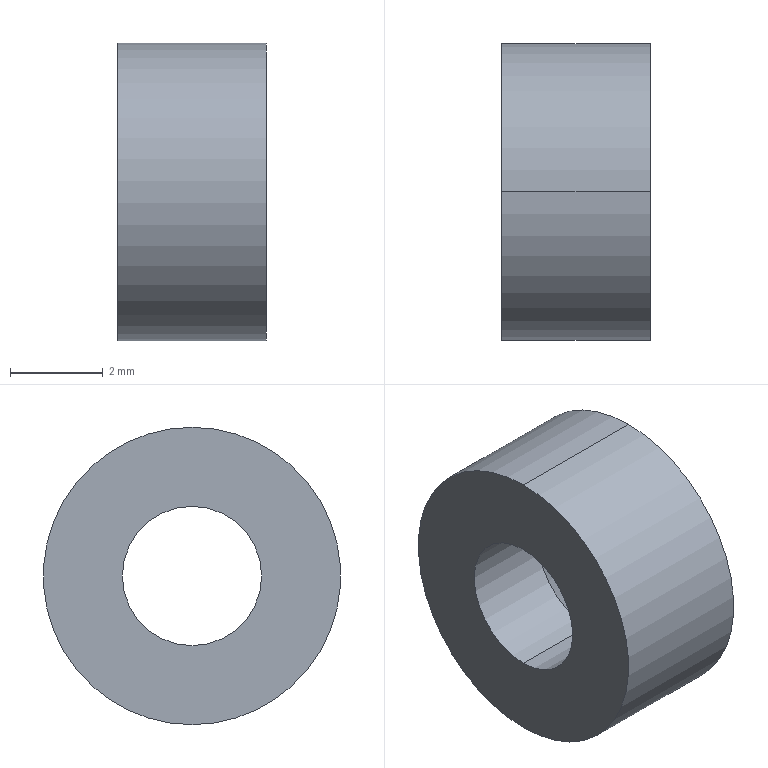Part | STEP file | 11-FG99-HXCC8magnet-V3.0-kkkkkk-998.11 | 1 solid | 8 faces | box 3.2 x 6.4 x 6.4 mm | volume 70.916 mm3 | cylinder 4 | cone 2 | plane 2 | commonest cylinder face diameters 3 x2 6.4 x2
STEP:
#1=CARTESIAN_POINT('',(3.8,0.,3.2));
#2=VERTEX_POINT('',#1);
#3=CARTESIAN_POINT('',(3.8,0.,-3.2));
#4=VERTEX_POINT('',#3);
#5=CARTESIAN_POINT('',(3.8,0.,0.));
#6=DIRECTION('',(-1.,0.,0.));
#7=DIRECTION('',(0.,0.,1.));
#8=AXIS2_PLACEMENT_3D('',#5,#6,#7);
#9=CIRCLE('',#8,3.2);
#10=EDGE_CURVE('',#2,#4,#9,.T.);
#11=ORIENTED_EDGE('',*,*,#10,.T.);
#12=CARTESIAN_POINT('',(0.6,0.,-3.2));
#13=VERTEX_POINT('',#12);
#14=CARTESIAN_POINT('',(4.,0.,-3.2));
#15=DIRECTION('',(-1.,0.,0.));
#16=VECTOR('',#15,1000.);
#17=LINE('',#14,#16);
#18=EDGE_CURVE('',#4,#13,#17,.T.);
#19=ORIENTED_EDGE('',*,*,#18,.T.);
#20=CARTESIAN_POINT('',(0.6,0.,3.2));
#21=VERTEX_POINT('',#20);
#22=CARTESIAN_POINT('',(0.6,0.,0.));
#23=DIRECTION('',(-1.,0.,0.));
#24=DIRECTION('',(0.,0.,1.));
#25=AXIS2_PLACEMENT_3D('',#22,#23,#24);
#26=CIRCLE('',#25,3.2);
#27=EDGE_CURVE('',#21,#13,#26,.T.);
#28=ORIENTED_EDGE('',*,*,#27,.F.);
#29=CARTESIAN_POINT('',(4.,0.,3.2));
#30=DIRECTION('',(-1.,0.,0.));
#31=VECTOR('',#30,1000.);
#32=LINE('',#29,#31);
#33=EDGE_CURVE('',#2,#21,#32,.T.);
#34=ORIENTED_EDGE('',*,*,#33,.F.);
#35=EDGE_LOOP('',(#11,#19,#28,#34));
#36=FACE_OUTER_BOUND('',#35,.T.);
#37=CARTESIAN_POINT('',(4.,0.,0.));
#38=DIRECTION('',(-1.,0.,0.));
#39=DIRECTION('',(0.,0.,1.));
#40=AXIS2_PLACEMENT_3D('',#37,#38,#39);
#41=CYLINDRICAL_SURFACE('',#40,3.2);
#42=ADVANCED_FACE('',(#36),#41,.T.);
#43=CARTESIAN_POINT('',(2.55,0.,-1.5));
#44=VERTEX_POINT('',#43);
#45=CARTESIAN_POINT('',(2.55,0.,1.5));
#46=VERTEX_POINT('',#45);
#47=CARTESIAN_POINT('',(2.55,0.,0.));
#48=DIRECTION('',(-1.,0.,0.));
#49=DIRECTION('',(0.,0.,1.));
#50=AXIS2_PLACEMENT_3D('',#47,#48,#49);
#51=CIRCLE('',#50,1.5);
#52=EDGE_CURVE('',#44,#46,#51,.T.);
#53=ORIENTED_EDGE('',*,*,#52,.T.);
#54=CARTESIAN_POINT('',(3.8,0.,2.75));
#55=VERTEX_POINT('',#54);
#56=CARTESIAN_POINT('',(2.55,0.,1.5));
#57=DIRECTION('',(0.7071,0.,0.7071));
#58=VECTOR('',#57,1000.);
#59=LINE('',#56,#58);
#60=EDGE_CURVE('',#46,#55,#59,.T.);
#61=ORIENTED_EDGE('',*,*,#60,.T.);
#62=CARTESIAN_POINT('',(3.8,0.,-2.75));
#63=VERTEX_POINT('',#62);
#64=CARTESIAN_POINT('',(3.8,0.,0.));
#65=DIRECTION('',(-1.,0.,0.));
#66=DIRECTION('',(0.,0.,1.));
#67=AXIS2_PLACEMENT_3D('',#64,#65,#66);
#68=CIRCLE('',#67,2.75);
#69=EDGE_CURVE('',#63,#55,#68,.T.);
#70=ORIENTED_EDGE('',*,*,#69,.F.);
#71=CARTESIAN_POINT('',(2.55,0.,-1.5));
#72=DIRECTION('',(0.7071,0.,-0.7071));
#73=VECTOR('',#72,1000.);
#74=LINE('',#71,#73);
#75=EDGE_CURVE('',#44,#63,#74,.T.);
#76=ORIENTED_EDGE('',*,*,#75,.F.);
#77=EDGE_LOOP('',(#53,#61,#70,#76));
#78=FACE_OUTER_BOUND('',#77,.T.);
#79=CARTESIAN_POINT('',(2.55,0.,0.));
#80=DIRECTION('',(1.,0.,0.));
#81=DIRECTION('',(0.,0.,-1.));
#82=AXIS2_PLACEMENT_3D('',#79,#80,#81);
#83=CONICAL_SURFACE('',#82,1.5,0.7854);
#84=ADVANCED_FACE('',(#78),#83,.F.);
#85=ORIENTED_EDGE('',*,*,#52,.F.);
#86=CARTESIAN_POINT('',(0.6,0.,-1.5));
#87=VERTEX_POINT('',#86);
#88=CARTESIAN_POINT('',(4.,0.,-1.5));
#89=DIRECTION('',(-1.,0.,0.));
#90=VECTOR('',#89,1000.);
#91=LINE('',#88,#90);
#92=EDGE_CURVE('',#44,#87,#91,.T.);
#93=ORIENTED_EDGE('',*,*,#92,.T.);
#94=CARTESIAN_POINT('',(0.6,0.,1.5));
#95=VERTEX_POINT('',#94);
#96=CARTESIAN_POINT('',(0.6,0.,0.));
#97=DIRECTION('',(-1.,0.,0.));
#98=DIRECTION('',(0.,0.,1.));
#99=AXIS2_PLACEMENT_3D('',#96,#97,#98);
#100=CIRCLE('',#99,1.5);
#101=EDGE_CURVE('',#87,#95,#100,.T.);
#102=ORIENTED_EDGE('',*,*,#101,.T.);
#103=CARTESIAN_POINT('',(4.,0.,1.5));
#104=DIRECTION('',(-1.,0.,0.));
#105=VECTOR('',#104,1000.);
#106=LINE('',#103,#105);
#107=EDGE_CURVE('',#46,#95,#106,.T.);
#108=ORIENTED_EDGE('',*,*,#107,.F.);
#109=EDGE_LOOP('',(#85,#93,#102,#108));
#110=FACE_OUTER_BOUND('',#109,.T.);
#111=CARTESIAN_POINT('',(4.,0.,0.));
#112=DIRECTION('',(-1.,0.,0.));
#113=DIRECTION('',(0.,0.,1.));
#114=AXIS2_PLACEMENT_3D('',#111,#112,#113);
#115=CYLINDRICAL_SURFACE('',#114,1.5);
#116=ADVANCED_FACE('',(#110),#115,.F.);
#117=CARTESIAN_POINT('',(0.6,0.,0.));
#118=DIRECTION('',(-1.,0.,0.));
#119=DIRECTION('',(0.,0.,1.));
#120=AXIS2_PLACEMENT_3D('',#117,#118,#119);
#121=CIRCLE('',#120,1.5);
#122=EDGE_CURVE('',#95,#87,#121,.T.);
#123=ORIENTED_EDGE('',*,*,#122,.F.);
#124=ORIENTED_EDGE('',*,*,#101,.F.);
#125=EDGE_LOOP('',(#123,#124));
#126=FACE_BOUND('',#125,.T.);
#127=ORIENTED_EDGE('',*,*,#27,.T.);
#128=CARTESIAN_POINT('',(0.6,0.,0.));
#129=DIRECTION('',(-1.,0.,0.));
#130=DIRECTION('',(0.,0.,1.));
#131=AXIS2_PLACEMENT_3D('',#128,#129,#130);
#132=CIRCLE('',#131,3.2);
#133=EDGE_CURVE('',#13,#21,#132,.T.);
#134=ORIENTED_EDGE('',*,*,#133,.T.);
#135=EDGE_LOOP('',(#127,#134));
#136=FACE_OUTER_BOUND('',#135,.T.);
#137=CARTESIAN_POINT('',(0.6,3.2,0.));
#138=DIRECTION('',(1.,0.,0.));
#139=DIRECTION('',(0.,0.,-1.));
#140=AXIS2_PLACEMENT_3D('',#137,#138,#139);
#141=PLANE('',#140);
#142=ADVANCED_FACE('',(#126,#136),#141,.F.);
#143=ORIENTED_EDGE('',*,*,#92,.F.);
#144=CARTESIAN_POINT('',(2.55,0.,0.));
#145=DIRECTION('',(-1.,0.,0.));
#146=DIRECTION('',(0.,0.,1.));
#147=AXIS2_PLACEMENT_3D('',#144,#145,#146);
#148=CIRCLE('',#147,1.5);
#149=EDGE_CURVE('',#46,#44,#148,.T.);
#150=ORIENTED_EDGE('',*,*,#149,.F.);
#151=ORIENTED_EDGE('',*,*,#107,.T.);
#152=ORIENTED_EDGE('',*,*,#122,.T.);
#153=EDGE_LOOP('',(#143,#150,#151,#152));
#154=FACE_OUTER_BOUND('',#153,.T.);
#155=CARTESIAN_POINT('',(4.,0.,0.));
#156=DIRECTION('',(-1.,0.,0.));
#157=DIRECTION('',(0.,0.,1.));
#158=AXIS2_PLACEMENT_3D('',#155,#156,#157);
#159=CYLINDRICAL_SURFACE('',#158,1.5);
#160=ADVANCED_FACE('',(#154),#159,.F.);
#161=ORIENTED_EDGE('',*,*,#60,.F.);
#162=ORIENTED_EDGE('',*,*,#149,.T.);
#163=ORIENTED_EDGE('',*,*,#75,.T.);
#164=CARTESIAN_POINT('',(3.8,0.,0.));
#165=DIRECTION('',(-1.,0.,0.));
#166=DIRECTION('',(0.,0.,1.));
#167=AXIS2_PLACEMENT_3D('',#164,#165,#166);
#168=CIRCLE('',#167,2.75);
#169=EDGE_CURVE('',#55,#63,#168,.T.);
#170=ORIENTED_EDGE('',*,*,#169,.F.);
#171=EDGE_LOOP('',(#161,#162,#163,#170));
#172=FACE_OUTER_BOUND('',#171,.T.);
#173=CARTESIAN_POINT('',(2.55,0.,0.));
#174=DIRECTION('',(1.,0.,0.));
#175=DIRECTION('',(0.,0.,-1.));
#176=AXIS2_PLACEMENT_3D('',#173,#174,#175);
#177=CONICAL_SURFACE('',#176,1.5,0.7854);
#178=ADVANCED_FACE('',(#172),#177,.F.);
#179=ORIENTED_EDGE('',*,*,#10,.F.);
#180=CARTESIAN_POINT('',(3.8,0.,0.));
#181=DIRECTION('',(-1.,0.,0.));
#182=DIRECTION('',(0.,0.,1.));
#183=AXIS2_PLACEMENT_3D('',#180,#181,#182);
#184=CIRCLE('',#183,3.2);
#185=EDGE_CURVE('',#4,#2,#184,.T.);
#186=ORIENTED_EDGE('',*,*,#185,.F.);
#187=EDGE_LOOP('',(#179,#186));
#188=FACE_OUTER_BOUND('',#187,.T.);
#189=ORIENTED_EDGE('',*,*,#69,.T.);
#190=ORIENTED_EDGE('',*,*,#169,.T.);
#191=EDGE_LOOP('',(#189,#190));
#192=FACE_BOUND('',#191,.T.);
#193=CARTESIAN_POINT('',(3.8,2.75,0.));
#194=DIRECTION('',(-1.,0.,0.));
#195=DIRECTION('',(0.,0.,1.));
#196=AXIS2_PLACEMENT_3D('',#193,#194,#195);
#197=PLANE('',#196);
#198=ADVANCED_FACE('',(#188,#192),#197,.F.);
#199=ORIENTED_EDGE('',*,*,#18,.F.);
#200=ORIENTED_EDGE('',*,*,#185,.T.);
#201=ORIENTED_EDGE('',*,*,#33,.T.);
#202=ORIENTED_EDGE('',*,*,#133,.F.);
#203=EDGE_LOOP('',(#199,#200,#201,#202));
#204=FACE_OUTER_BOUND('',#203,.T.);
#205=CARTESIAN_POINT('',(4.,0.,0.));
#206=DIRECTION('',(-1.,0.,0.));
#207=DIRECTION('',(0.,0.,1.));
#208=AXIS2_PLACEMENT_3D('',#205,#206,#207);
#209=CYLINDRICAL_SURFACE('',#208,3.2);
#210=ADVANCED_FACE('',(#204),#209,.T.);
#211=CLOSED_SHELL('',(#42,#84,#116,#142,#160,#178,#198,#210));
#212=MANIFOLD_SOLID_BREP('',#211);
#213=CARTESIAN_POINT('',(0.,0.,0.));
#214=DIRECTION('',(0.,0.,1.));
#215=DIRECTION('',(1.,0.,0.));
#216=AXIS2_PLACEMENT_3D('',#213,#214,#215);
#217=(LENGTH_UNIT()NAMED_UNIT(*)SI_UNIT(.MILLI.,.METRE.));
#218=UNCERTAINTY_MEASURE_WITH_UNIT(LENGTH_MEASURE(0.00001),#217,'','');
#219=(NAMED_UNIT(*)PLANE_ANGLE_UNIT()SI_UNIT($,.RADIAN.));
#220=(NAMED_UNIT(*)SI_UNIT($,.STERADIAN.)SOLID_ANGLE_UNIT());
#221=(GEOMETRIC_REPRESENTATION_CONTEXT(3)GLOBAL_UNCERTAINTY_ASSIGNED_CONTEXT((#218))GLOBAL_UNIT_ASSIGNED_CONTEXT((#217,#219,#220))REPRESENTATION_CONTEXT('',''));
#222=ADVANCED_BREP_SHAPE_REPRESENTATION('',(#212,#216),#221);